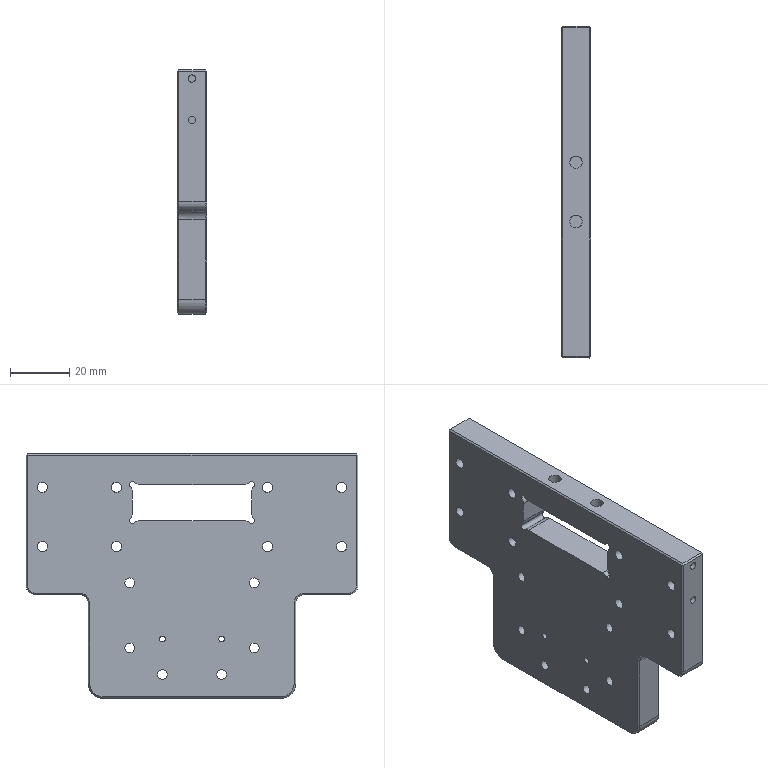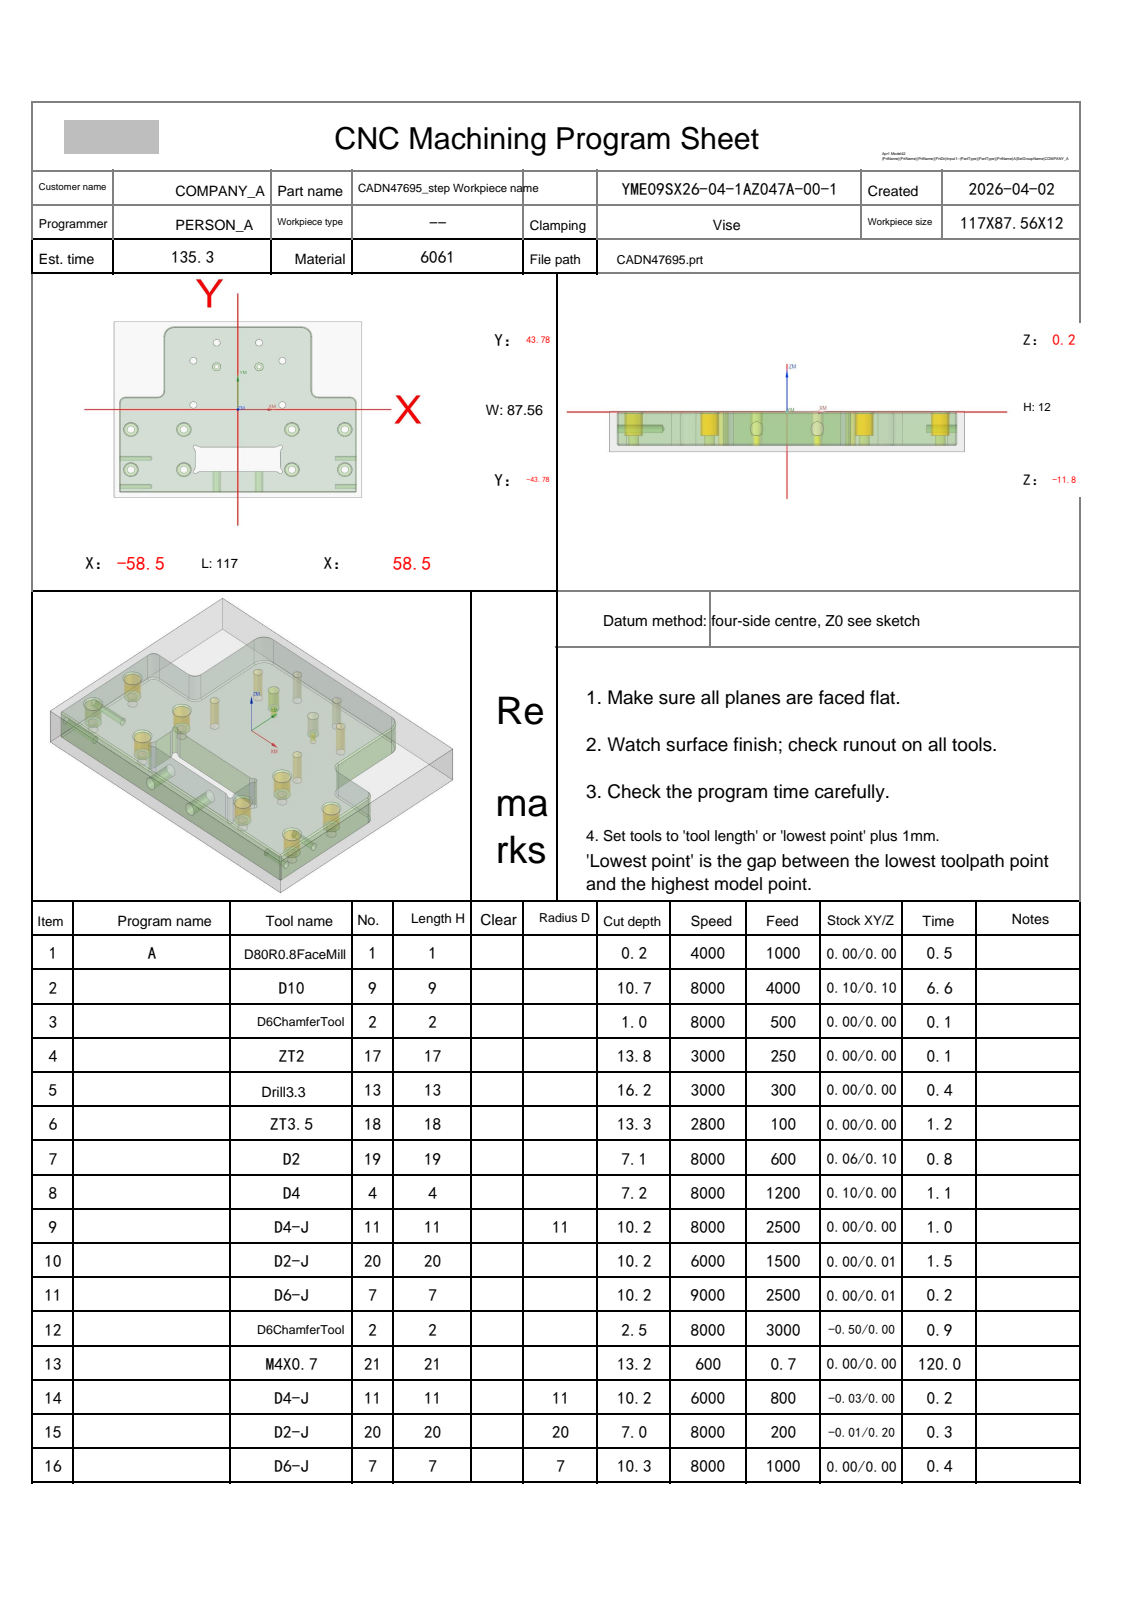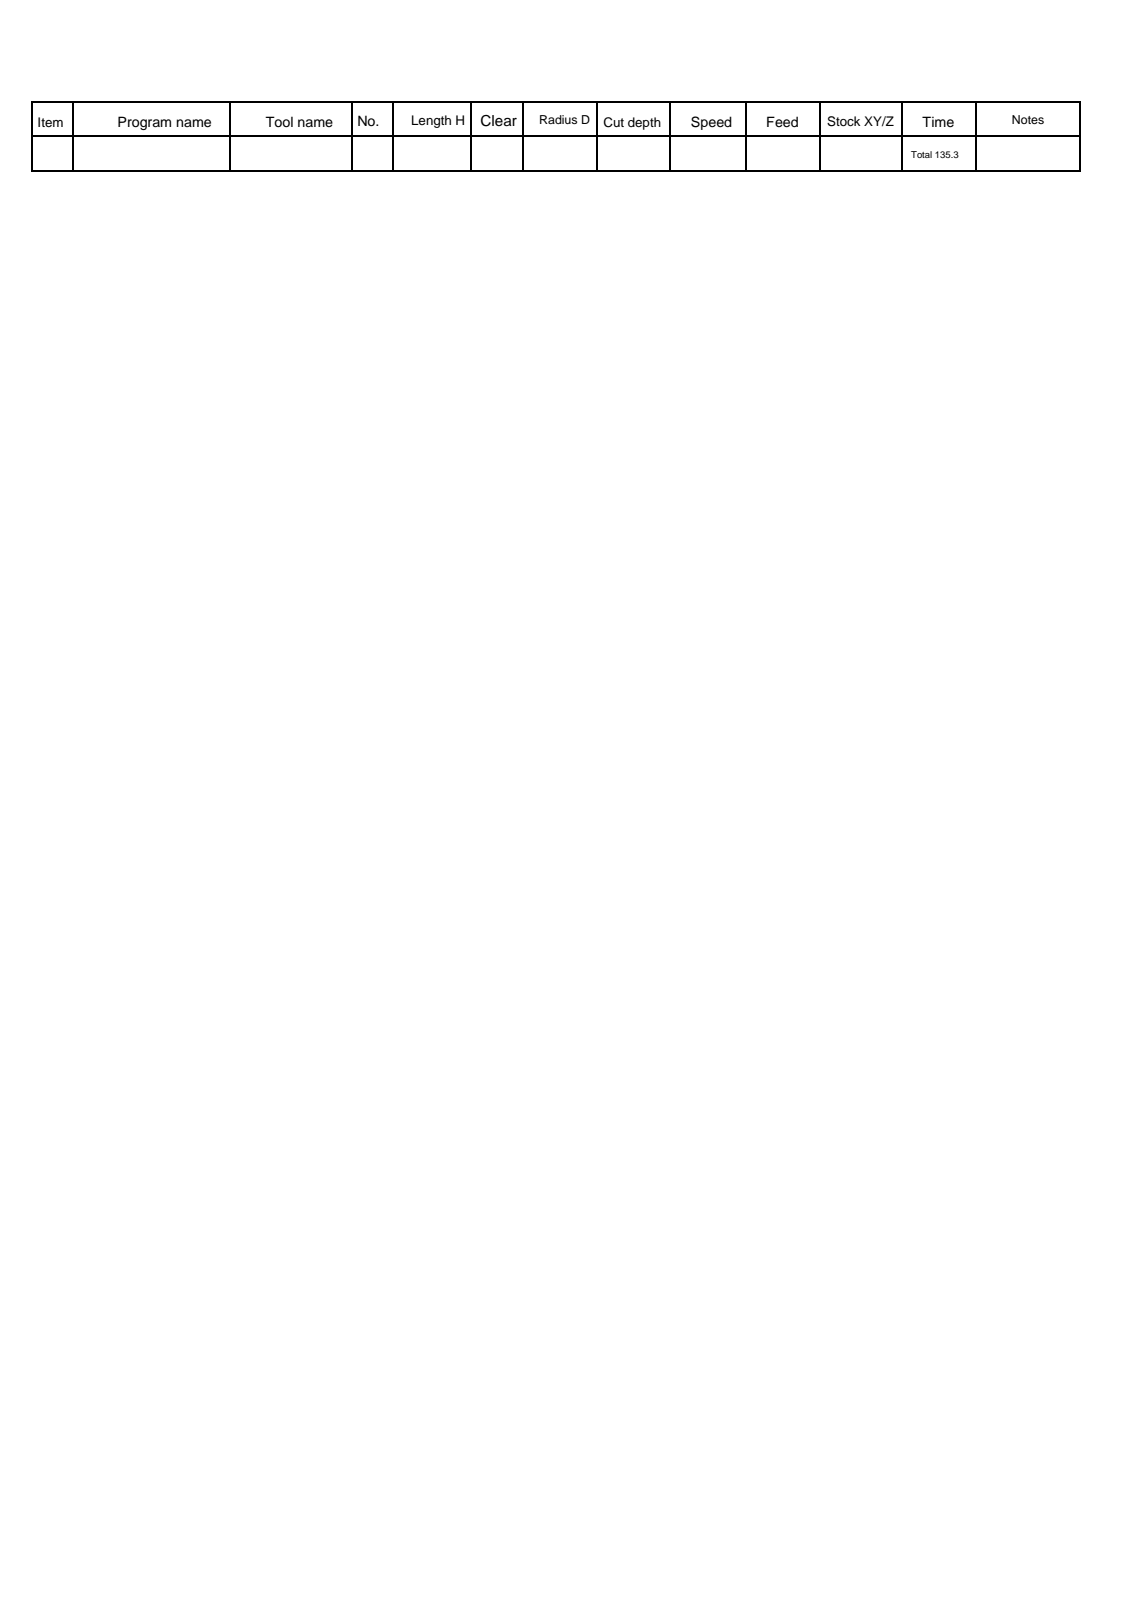NC program | NX | posted by the shop | part box 10 x 112 x 82.562 mm
Lines 3038 to 4053 of 16718:
N9 T11 M06
(D4-J  D=4. R=0. H=11 ce=0.00 di=0.00)
G00 G90 G54 X-50.5 Y-29.931 M03 S8000
G43 H11 Z20.
M08
Z.5
G41 D11
G01 X-50.577 Y-29.747 F500.
G03 X-51.02 Y-29.451 I-.443 J-.185
X-51.5 Y-29.931 I0.0 J-.48
X-51.5 Y-29.931 Z-4.5 I1. J0.0
X-49.5 Y-29.931 Z-7. I1. J0.0
X-50.5 Y-28.931 I-1. J0.0
X-51.5 Y-29.931 I0.0 J-1.
X-50.5 Y-30.931 I1. J0.0
X-49.5 Y-29.931 I0.0 J1.
X-49.98 Y-29.451 I-.48 J0.0
X-50.423 Y-29.747 I0.0 J-.48
G01 G40 X-50.5 Y-29.931
G00 Z20.
Y-9.931
Z.5
G41 D11
G01 X-50.577 Y-9.747
G03 X-51.02 Y-9.451 I-.443 J-.185
X-51.5 Y-9.931 I0.0 J-.48
X-51.5 Y-9.931 Z-4.5 I1. J0.0
X-49.5 Y-9.931 Z-7. I1. J0.0
X-50.5 Y-8.931 I-1. J0.0
X-51.5 Y-9.931 I0.0 J-1.
X-50.5 Y-10.931 I1. J0.0
X-49.5 Y-9.931 I0.0 J1.
X-49.98 Y-9.451 I-.48 J0.0
X-50.423 Y-9.747 I0.0 J-.48
G01 G40 X-50.5 Y-9.931
G00 Z20.
X-25.5
Z.5
G41 D11
G01 X-25.577 Y-9.747
G03 X-26.02 Y-9.451 I-.443 J-.185
X-26.5 Y-9.931 I0.0 J-.48
X-26.5 Y-9.931 Z-4.5 I1. J0.0
X-24.5 Y-9.931 Z-7. I1. J0.0
X-25.5 Y-8.931 I-1. J0.0
X-26.5 Y-9.931 I0.0 J-1.
X-25.5 Y-10.931 I1. J0.0
X-24.5 Y-9.931 I0.0 J1.
X-24.98 Y-9.451 I-.48 J0.0
X-25.423 Y-9.747 I0.0 J-.48
G01 G40 X-25.5 Y-9.931
G00 Z20.
Y-29.931
Z.5
G41 D11
G01 X-25.577 Y-29.747
G03 X-26.02 Y-29.451 I-.443 J-.185
X-26.5 Y-29.931 I0.0 J-.48
X-26.5 Y-29.931 Z-4.5 I1. J0.0
X-24.5 Y-29.931 Z-7. I1. J0.0
X-25.5 Y-28.931 I-1. J0.0
X-26.5 Y-29.931 I0.0 J-1.
X-25.5 Y-30.931 I1. J0.0
X-24.5 Y-29.931 I0.0 J1.
X-24.98 Y-29.451 I-.48 J0.0
X-25.423 Y-29.747 I0.0 J-.48
G01 G40 X-25.5 Y-29.931
G00 Z20.
X25.5
Z.5
G41 D11
G01 X25.423 Y-29.747
G03 X24.98 Y-29.451 I-.443 J-.185
X24.5 Y-29.931 I0.0 J-.48
X24.5 Y-29.931 Z-4.5 I1. J0.0
X26.5 Y-29.931 Z-7. I1. J0.0
X25.5 Y-28.931 I-1. J0.0
X24.5 Y-29.931 I0.0 J-1.
X25.5 Y-30.931 I1. J0.0
X26.5 Y-29.931 I0.0 J1.
X26.02 Y-29.451 I-.48 J0.0
X25.577 Y-29.747 I0.0 J-.48
G01 G40 X25.5 Y-29.931
G00 Z20.
Y-9.931
Z.5
G41 D11
G01 X25.423 Y-9.747
G03 X24.98 Y-9.451 I-.443 J-.185
X24.5 Y-9.931 I0.0 J-.48
X24.5 Y-9.931 Z-4.5 I1. J0.0
X26.5 Y-9.931 Z-7. I1. J0.0
X25.5 Y-8.931 I-1. J0.0
X24.5 Y-9.931 I0.0 J-1.
X25.5 Y-10.931 I1. J0.0
X26.5 Y-9.931 I0.0 J1.
X26.02 Y-9.451 I-.48 J0.0
X25.577 Y-9.747 I0.0 J-.48
G01 G40 X25.5 Y-9.931
G00 Z20.
X50.5
Z.5
G41 D11
G01 X50.423 Y-9.747
G03 X49.98 Y-9.451 I-.443 J-.185
X49.5 Y-9.931 I0.0 J-.48
X49.5 Y-9.931 Z-4.5 I1. J0.0
X51.5 Y-9.931 Z-7. I1. J0.0
X50.5 Y-8.931 I-1. J0.0
X49.5 Y-9.931 I0.0 J-1.
X50.5 Y-10.931 I1. J0.0
X51.5 Y-9.931 I0.0 J1.
X51.02 Y-9.451 I-.48 J0.0
X50.577 Y-9.747 I0.0 J-.48
G01 G40 X50.5 Y-9.931
G00 Z20.
Y-29.931
Z.5
G41 D11
G01 X50.423 Y-29.747
G03 X49.98 Y-29.451 I-.443 J-.185
X49.5 Y-29.931 I0.0 J-.48
X49.5 Y-29.931 Z-4.5 I1. J0.0
X51.5 Y-29.931 Z-7. I1. J0.0
X50.5 Y-28.931 I-1. J0.0
X49.5 Y-29.931 I0.0 J-1.
X50.5 Y-30.931 I1. J0.0
X51.5 Y-29.931 I0.0 J1.
X51.02 Y-29.451 I-.48 J0.0
X50.577 Y-29.747 I0.0 J-.48
G01 G40 X50.5 Y-29.931
G00 Z20.
G00 G90 X14.547 Y-28.28 M03 S6000
Z20.
Z.306
G01 X14.548 Y-28.287 Z.22 F2000.
X14.551 Y-28.306 Z.142
X14.556 Y-28.335 Z.072
X14.564 Y-28.374 Z.01
X14.575 Y-28.419 Z-.046
X14.589 Y-28.47 Z-.095
X14.606 Y-28.525 Z-.137
X14.627 Y-28.581 Z-.174
X14.651 Y-28.637 Z-.205
X14.68 Y-28.691 Z-.231
X14.712 Y-28.742 Z-.252
X14.749 Y-28.787 Z-.268
X14.791 Y-28.826 Z-.28
X14.838 Y-28.855 Z-.288
X14.89 Y-28.874 Z-.293
X14.947 Y-28.881 Z-.294
X17.651 F2500.
G02 X18.125 Y-28.906 I0.0 J-4.5
X18.1 Y-28.432 I4.475 J.475
G01 Y-25.728
X18.084 Y-25.685 Z-.295
X18.038 Y-25.664 Z-.298
X17.966 Y-25.663 Z-.302
X17.87 Y-25.681 Z-.307
X17.755 Y-25.716 Z-.314
X17.624 Y-25.766 Z-.322
X17.48 Y-25.83 Z-.331
X17.327 Y-25.905 Z-.341
X17.086 Y-26.039 Z-.357
X16.847 Y-26.187 Z-.374
X16.509 Y-26.429 Z-.4
X16.194 Y-26.696 Z-.427
X15.903 Y-26.986 Z-.455
X15.636 Y-27.3 Z-.482
X15.395 Y-27.636 Z-.509
X15.294 Y-27.795 Z-.52
X15.201 Y-27.956 Z-.531
X15.116 Y-28.114 Z-.542
X15.042 Y-28.266 Z-.551
X14.98 Y-28.408 Z-.56
X14.931 Y-28.539 Z-.568
X14.897 Y-28.653 Z-.575
X14.881 Y-28.748 Z-.581
X14.882 Y-28.82 Z-.585
X14.904 Y-28.865 Z-.587
X14.947 Y-28.881 Z-.588
X17.651
G02 X18.125 Y-28.906 I0.0 J-4.5
X18.1 Y-28.432 I4.475 J.475
G01 Y-25.728
X18.084 Y-25.685 Z-.589
X18.038 Y-25.664 Z-.592
X17.966 Y-25.663 Z-.596
X17.87 Y-25.681 Z-.601
X17.755 Y-25.716 Z-.608
X17.624 Y-25.766 Z-.616
X17.48 Y-25.83 Z-.625
X17.327 Y-25.905 Z-.635
X17.086 Y-26.039 Z-.651
X16.847 Y-26.187 Z-.668
X16.509 Y-26.429 Z-.694
X16.194 Y-26.696 Z-.722
X15.903 Y-26.986 Z-.749
X15.636 Y-27.3 Z-.776
X15.395 Y-27.636 Z-.803
X15.294 Y-27.795 Z-.814
X15.201 Y-27.956 Z-.825
X15.116 Y-28.114 Z-.836
X15.042 Y-28.266 Z-.846
X14.98 Y-28.408 Z-.855
X14.931 Y-28.539 Z-.862
X14.897 Y-28.653 Z-.869
X14.881 Y-28.748 Z-.875
X14.882 Y-28.82 Z-.879
X14.904 Y-28.865 Z-.881
X14.947 Y-28.881 Z-.882
X17.651
G02 X18.125 Y-28.906 I0.0 J-4.5
X18.1 Y-28.432 I4.475 J.475
G01 Y-25.728
X18.084 Y-25.685 Z-.883
X18.038 Y-25.664 Z-.886
X17.966 Y-25.663 Z-.89
X17.87 Y-25.681 Z-.895
X17.755 Y-25.716 Z-.902
X17.624 Y-25.766 Z-.91
X17.48 Y-25.83 Z-.919
X17.327 Y-25.905 Z-.929
X17.086 Y-26.039 Z-.945
X16.847 Y-26.187 Z-.962
X16.509 Y-26.429 Z-.988
X16.194 Y-26.696 Z-1.016
X15.903 Y-26.986 Z-1.043
X15.636 Y-27.3 Z-1.07
X15.395 Y-27.636 Z-1.097
X15.294 Y-27.795 Z-1.108
X15.201 Y-27.956 Z-1.119
X15.116 Y-28.114 Z-1.13
X15.042 Y-28.266 Z-1.14
X14.98 Y-28.408 Z-1.149
X14.931 Y-28.539 Z-1.157
X14.897 Y-28.653 Z-1.163
X14.881 Y-28.748 Z-1.169
X14.882 Y-28.82 Z-1.173
X14.904 Y-28.865 Z-1.176
X14.947 Y-28.881
X17.651
G02 X18.125 Y-28.906 I0.0 J-4.5
X18.1 Y-28.432 I4.475 J.475
G01 Y-25.728
X18.084 Y-25.685 Z-1.177
X18.038 Y-25.664 Z-1.18
X17.966 Y-25.663 Z-1.184
X17.87 Y-25.681 Z-1.19
X17.755 Y-25.716 Z-1.196
X17.624 Y-25.766 Z-1.204
X17.48 Y-25.83 Z-1.213
X17.327 Y-25.905 Z-1.223
X17.086 Y-26.039 Z-1.239
X16.847 Y-26.187 Z-1.256
X16.509 Y-26.429 Z-1.283
X16.194 Y-26.696 Z-1.31
X15.903 Y-26.986 Z-1.337
X15.636 Y-27.3 Z-1.365
X15.395 Y-27.636 Z-1.391
X15.294 Y-27.795 Z-1.402
X15.201 Y-27.956 Z-1.414
X15.116 Y-28.114 Z-1.424
X15.042 Y-28.266 Z-1.434
X14.98 Y-28.408 Z-1.443
X14.931 Y-28.539 Z-1.451
X14.897 Y-28.653 Z-1.457
X14.881 Y-28.748 Z-1.463
X14.882 Y-28.82 Z-1.467
X14.904 Y-28.865 Z-1.47
X14.947 Y-28.881 Z-1.471
X17.651
G02 X18.125 Y-28.906 I0.0 J-4.5
X18.1 Y-28.432 I4.475 J.475
G01 Y-25.728
X18.084 Y-25.685
X18.038 Y-25.664 Z-1.474
X17.966 Y-25.663 Z-1.478
X17.87 Y-25.681 Z-1.484
X17.755 Y-25.716 Z-1.491
X17.624 Y-25.766 Z-1.498
X17.48 Y-25.83 Z-1.507
X17.327 Y-25.905 Z-1.517
X17.086 Y-26.039 Z-1.533
X16.847 Y-26.187 Z-1.55
X16.509 Y-26.429 Z-1.577
X16.194 Y-26.696 Z-1.604
X15.903 Y-26.986 Z-1.631
X15.636 Y-27.3 Z-1.659
X15.395 Y-27.636 Z-1.685
X15.294 Y-27.795 Z-1.697
X15.201 Y-27.956 Z-1.708
X15.116 Y-28.114 Z-1.718
X15.042 Y-28.266 Z-1.728
X14.98 Y-28.408 Z-1.737
X14.931 Y-28.539 Z-1.745
X14.897 Y-28.653 Z-1.752
X14.881 Y-28.748 Z-1.757
X14.882 Y-28.82 Z-1.761
X14.904 Y-28.865 Z-1.764
X14.947 Y-28.881 Z-1.765
X17.651
G02 X18.125 Y-28.906 I0.0 J-4.5
X18.1 Y-28.432 I4.475 J.475
G01 Y-25.728
X18.084 Y-25.685 Z-1.766
X18.038 Y-25.664 Z-1.768
X17.966 Y-25.663 Z-1.772
X17.87 Y-25.681 Z-1.778
X17.755 Y-25.716 Z-1.785
X17.624 Y-25.766 Z-1.793
X17.48 Y-25.83 Z-1.801
X17.327 Y-25.905 Z-1.811
X17.086 Y-26.039 Z-1.827
X16.847 Y-26.187 Z-1.844
X16.509 Y-26.429 Z-1.871
X16.194 Y-26.696 Z-1.898
X15.903 Y-26.986 Z-1.926
X15.636 Y-27.3 Z-1.953
X15.395 Y-27.636 Z-1.979
X15.294 Y-27.795 Z-1.991
X15.201 Y-27.956 Z-2.002
X15.116 Y-28.114 Z-2.012
X15.042 Y-28.266 Z-2.022
X14.98 Y-28.408 Z-2.031
X14.931 Y-28.539 Z-2.039
X14.897 Y-28.653 Z-2.046
X14.881 Y-28.748 Z-2.051
X14.882 Y-28.82 Z-2.055
X14.904 Y-28.865 Z-2.058
X14.947 Y-28.881 Z-2.059
X17.651
G02 X18.125 Y-28.906 I0.0 J-4.5
X18.1 Y-28.432 I4.475 J.475
G01 Y-25.728
X18.084 Y-25.685 Z-2.06
X18.038 Y-25.664 Z-2.062
X17.966 Y-25.663 Z-2.066
X17.87 Y-25.681 Z-2.072
X17.755 Y-25.716 Z-2.079
X17.624 Y-25.766 Z-2.087
X17.48 Y-25.83 Z-2.096
X17.327 Y-25.905 Z-2.105
X17.086 Y-26.039 Z-2.122
X16.847 Y-26.187 Z-2.138
X16.509 Y-26.429 Z-2.165
X16.194 Y-26.696 Z-2.192
X15.903 Y-26.986 Z-2.22
X15.636 Y-27.3 Z-2.247
X15.395 Y-27.636 Z-2.273
X15.294 Y-27.795 Z-2.285
X15.201 Y-27.956 Z-2.296
X15.116 Y-28.114 Z-2.306
X15.042 Y-28.266 Z-2.316
X14.98 Y-28.408 Z-2.325
X14.931 Y-28.539 Z-2.333
X14.897 Y-28.653 Z-2.34
X14.881 Y-28.748 Z-2.345
X14.882 Y-28.82 Z-2.349
X14.904 Y-28.865 Z-2.352
X14.947 Y-28.881 Z-2.353
X17.651
G02 X18.125 Y-28.906 I0.0 J-4.5
X18.1 Y-28.432 I4.475 J.475
G01 Y-25.728
X18.084 Y-25.685 Z-2.354
X18.038 Y-25.664 Z-2.356
X17.966 Y-25.663 Z-2.361
X17.87 Y-25.681 Z-2.366
X17.755 Y-25.716 Z-2.373
X17.624 Y-25.766 Z-2.381
X17.48 Y-25.83 Z-2.39
X17.327 Y-25.905 Z-2.399
X17.086 Y-26.039 Z-2.416
X16.847 Y-26.187 Z-2.433
X16.509 Y-26.429 Z-2.459
X16.194 Y-26.696 Z-2.486
X15.903 Y-26.986 Z-2.514
X15.636 Y-27.3 Z-2.541
X15.395 Y-27.636 Z-2.567
X15.294 Y-27.795 Z-2.579
X15.201 Y-27.956 Z-2.59
X15.116 Y-28.114 Z-2.601
X15.042 Y-28.266 Z-2.61
X14.98 Y-28.408 Z-2.619
X14.931 Y-28.539 Z-2.627
X14.897 Y-28.653 Z-2.634
X14.881 Y-28.748 Z-2.639
X14.882 Y-28.82 Z-2.644
X14.904 Y-28.865 Z-2.646
X14.947 Y-28.881 Z-2.647
X17.651
G02 X18.125 Y-28.906 I0.0 J-4.5
X18.1 Y-28.432 I4.475 J.475
G01 Y-25.728
X18.084 Y-25.685 Z-2.648
X18.038 Y-25.664 Z-2.651
X17.966 Y-25.663 Z-2.655
X17.87 Y-25.681 Z-2.66
X17.755 Y-25.716 Z-2.667
X17.624 Y-25.766 Z-2.675
X17.48 Y-25.83 Z-2.684
X17.327 Y-25.905 Z-2.694
X17.086 Y-26.039 Z-2.71
X16.847 Y-26.187 Z-2.727
X16.509 Y-26.429 Z-2.753
X16.194 Y-26.696 Z-2.78
X15.903 Y-26.986 Z-2.808
X15.636 Y-27.3 Z-2.835
X15.395 Y-27.636 Z-2.862
X15.294 Y-27.795 Z-2.873
X15.201 Y-27.956 Z-2.884
X15.116 Y-28.114 Z-2.895
X15.042 Y-28.266 Z-2.904
X14.98 Y-28.408 Z-2.913
X14.931 Y-28.539 Z-2.921
X14.897 Y-28.653 Z-2.928
X14.881 Y-28.748 Z-2.934
X14.882 Y-28.82 Z-2.938
X14.904 Y-28.865 Z-2.94
X14.947 Y-28.881 Z-2.941
X17.651
G02 X18.125 Y-28.906 I0.0 J-4.5
X18.1 Y-28.432 I4.475 J.475
G01 Y-25.728
X18.084 Y-25.685 Z-2.942
X18.038 Y-25.664 Z-2.945
X17.966 Y-25.663 Z-2.949
X17.87 Y-25.681 Z-2.954
X17.755 Y-25.716 Z-2.961
X17.624 Y-25.766 Z-2.969
X17.48 Y-25.83 Z-2.978
X17.327 Y-25.905 Z-2.988
X17.086 Y-26.039 Z-3.004
X16.847 Y-26.187 Z-3.021
X16.509 Y-26.429 Z-3.047
X16.194 Y-26.696 Z-3.074
X15.903 Y-26.986 Z-3.102
X15.636 Y-27.3 Z-3.129
X15.395 Y-27.636 Z-3.156
X15.294 Y-27.795 Z-3.167
X15.201 Y-27.956 Z-3.178
X15.116 Y-28.114 Z-3.189
X15.042 Y-28.266 Z-3.199
X14.98 Y-28.408 Z-3.207
X14.931 Y-28.539 Z-3.215
X14.897 Y-28.653 Z-3.222
X14.881 Y-28.748 Z-3.228
X14.882 Y-28.82 Z-3.232
X14.904 Y-28.865 Z-3.234
X14.947 Y-28.881 Z-3.235
X17.651
G02 X18.125 Y-28.906 I0.0 J-4.5
X18.1 Y-28.432 I4.475 J.475
G01 Y-25.728
X18.084 Y-25.685 Z-3.236
X18.038 Y-25.664 Z-3.239
X17.966 Y-25.663 Z-3.243
X17.87 Y-25.681 Z-3.248
X17.755 Y-25.716 Z-3.255
X17.624 Y-25.766 Z-3.263
X17.48 Y-25.83 Z-3.272
X17.327 Y-25.905 Z-3.282
X17.086 Y-26.039 Z-3.298
X16.847 Y-26.187 Z-3.315
X16.509 Y-26.429 Z-3.341
X16.194 Y-26.696 Z-3.369
X15.903 Y-26.986 Z-3.396
X15.636 Y-27.3 Z-3.423
X15.395 Y-27.636 Z-3.45
X15.294 Y-27.795 Z-3.461
X15.201 Y-27.956 Z-3.472
X15.116 Y-28.114 Z-3.483
X15.042 Y-28.266 Z-3.493
X14.98 Y-28.408 Z-3.502
X14.931 Y-28.539 Z-3.51
X14.897 Y-28.653 Z-3.516
X14.881 Y-28.748 Z-3.522
X14.882 Y-28.82 Z-3.526
X14.904 Y-28.865 Z-3.529
X14.947 Y-28.881
X17.651
G02 X18.125 Y-28.906 I0.0 J-4.5
X18.1 Y-28.432 I4.475 J.475
G01 Y-25.728
X18.084 Y-25.685 Z-3.53
X18.038 Y-25.664 Z-3.533
X17.966 Y-25.663 Z-3.537
X17.87 Y-25.681 Z-3.543
X17.755 Y-25.716 Z-3.549
X17.624 Y-25.766 Z-3.557
X17.48 Y-25.83 Z-3.566
X17.327 Y-25.905 Z-3.576
X17.086 Y-26.039 Z-3.592
X16.847 Y-26.187 Z-3.609
X16.509 Y-26.429 Z-3.635
X16.194 Y-26.696 Z-3.663
X15.903 Y-26.986 Z-3.69
X15.636 Y-27.3 Z-3.718
X15.395 Y-27.636 Z-3.744
X15.294 Y-27.795 Z-3.755
X15.201 Y-27.956 Z-3.766
X15.116 Y-28.114 Z-3.777
X15.042 Y-28.266 Z-3.787
X14.98 Y-28.408 Z-3.796
X14.931 Y-28.539 Z-3.804
X14.897 Y-28.653 Z-3.81
X14.881 Y-28.748 Z-3.816
X14.882 Y-28.82 Z-3.82
X14.904 Y-28.865 Z-3.823
X14.947 Y-28.881 Z-3.824
X17.651
G02 X18.125 Y-28.906 I0.0 J-4.5
X18.1 Y-28.432 I4.475 J.475
G01 Y-25.728
X18.084 Y-25.685
X18.038 Y-25.664 Z-3.827
X17.966 Y-25.663 Z-3.831
X17.87 Y-25.681 Z-3.837
X17.755 Y-25.716 Z-3.843
X17.624 Y-25.766 Z-3.851
X17.48 Y-25.83 Z-3.86
X17.327 Y-25.905 Z-3.87
X17.086 Y-26.039 Z-3.886
X16.847 Y-26.187 Z-3.903
X16.509 Y-26.429 Z-3.93
X16.194 Y-26.696 Z-3.957
X15.903 Y-26.986 Z-3.984
X15.636 Y-27.3 Z-4.012
X15.395 Y-27.636 Z-4.038
X15.294 Y-27.795 Z-4.05
X15.201 Y-27.956 Z-4.061
X15.116 Y-28.114 Z-4.071
X15.042 Y-28.266 Z-4.081
X14.98 Y-28.408 Z-4.09
X14.931 Y-28.539 Z-4.098
X14.897 Y-28.653 Z-4.105
X14.881 Y-28.748 Z-4.11
X14.882 Y-28.82 Z-4.114
X14.904 Y-28.865 Z-4.117
X14.947 Y-28.881 Z-4.118
X17.651
G02 X18.125 Y-28.906 I0.0 J-4.5
X18.1 Y-28.432 I4.475 J.475
G01 Y-25.728
X18.084 Y-25.685 Z-4.119
X18.038 Y-25.664 Z-4.121
X17.966 Y-25.663 Z-4.125
X17.87 Y-25.681 Z-4.131
X17.755 Y-25.716 Z-4.138
X17.624 Y-25.766 Z-4.145
X17.48 Y-25.83 Z-4.154
X17.327 Y-25.905 Z-4.164
X17.086 Y-26.039 Z-4.18
X16.847 Y-26.187 Z-4.197
X16.509 Y-26.429 Z-4.224
X16.194 Y-26.696 Z-4.251
X15.903 Y-26.986 Z-4.278
X15.636 Y-27.3 Z-4.306
X15.395 Y-27.636 Z-4.332
X15.294 Y-27.795 Z-4.344
X15.201 Y-27.956 Z-4.355
X15.116 Y-28.114 Z-4.365
X15.042 Y-28.266 Z-4.375
X14.98 Y-28.408 Z-4.384
X14.931 Y-28.539 Z-4.392
X14.897 Y-28.653 Z-4.399
X14.881 Y-28.748 Z-4.404
X14.882 Y-28.82 Z-4.408
X14.904 Y-28.865 Z-4.411
X14.947 Y-28.881 Z-4.412
X17.651
G02 X18.125 Y-28.906 I0.0 J-4.5
X18.1 Y-28.432 I4.475 J.475
G01 Y-25.728
X18.084 Y-25.685 Z-4.413
X18.038 Y-25.664 Z-4.415
X17.966 Y-25.663 Z-4.419
X17.87 Y-25.681 Z-4.425
X17.755 Y-25.716 Z-4.432
X17.624 Y-25.766 Z-4.44
X17.48 Y-25.83 Z-4.449
X17.327 Y-25.905 Z-4.458
X17.086 Y-26.039 Z-4.474
X16.847 Y-26.187 Z-4.491
X16.509 Y-26.429 Z-4.518
X16.194 Y-26.696 Z-4.545
X15.903 Y-26.986 Z-4.573
X15.636 Y-27.3 Z-4.6
X15.395 Y-27.636 Z-4.626
X15.294 Y-27.795 Z-4.638
X15.201 Y-27.956 Z-4.649
X15.116 Y-28.114 Z-4.659
X15.042 Y-28.266 Z-4.669
X14.98 Y-28.408 Z-4.678
X14.931 Y-28.539 Z-4.686
X14.897 Y-28.653 Z-4.693
X14.881 Y-28.748 Z-4.698
X14.882 Y-28.82 Z-4.702
X14.904 Y-28.865 Z-4.705
X14.947 Y-28.881 Z-4.706
X17.651
G02 X18.125 Y-28.906 I0.0 J-4.5
X18.1 Y-28.432 I4.475 J.475
G01 Y-25.728
X18.084 Y-25.685 Z-4.707
X18.038 Y-25.664 Z-4.709
X17.966 Y-25.663 Z-4.713
X17.87 Y-25.681 Z-4.719
X17.755 Y-25.716 Z-4.726
X17.624 Y-25.766 Z-4.734
X17.48 Y-25.83 Z-4.743
X17.327 Y-25.905 Z-4.752
X17.086 Y-26.039 Z-4.769
X16.847 Y-26.187 Z-4.786
X16.509 Y-26.429 Z-4.812
X16.194 Y-26.696 Z-4.839
X15.903 Y-26.986 Z-4.867
X15.636 Y-27.3 Z-4.894
X15.395 Y-27.636 Z-4.92
X15.294 Y-27.795 Z-4.932
X15.201 Y-27.956 Z-4.943
X15.116 Y-28.114 Z-4.953
X15.042 Y-28.266 Z-4.963
X14.98 Y-28.408 Z-4.972
X14.931 Y-28.539 Z-4.98
X14.897 Y-28.653 Z-4.987
X14.881 Y-28.748 Z-4.992
X14.882 Y-28.82 Z-4.997
X14.904 Y-28.865 Z-4.999
X14.947 Y-28.881 Z-5.
X17.651
G02 X18.125 Y-28.906 I0.0 J-4.5
X18.1 Y-28.432 I4.475 J.475
G01 Y-25.728
X18.084 Y-25.685 Z-5.001
X18.038 Y-25.664 Z-5.003
X17.966 Y-25.663 Z-5.008
X17.87 Y-25.681 Z-5.013
X17.755 Y-25.716 Z-5.02
X17.624 Y-25.766 Z-5.028
X17.48 Y-25.83 Z-5.037
X17.327 Y-25.905 Z-5.047
X17.086 Y-26.039 Z-5.063
X16.847 Y-26.187 Z-5.08
X16.509 Y-26.429 Z-5.106
X16.194 Y-26.696 Z-5.133
X15.903 Y-26.986 Z-5.161
X15.636 Y-27.3 Z-5.188
X15.395 Y-27.636 Z-5.214
X15.294 Y-27.795 Z-5.226
X15.201 Y-27.956 Z-5.237
X15.116 Y-28.114 Z-5.248
X15.042 Y-28.266 Z-5.257
X14.98 Y-28.408 Z-5.266
X14.931 Y-28.539 Z-5.274
X14.897 Y-28.653 Z-5.281
X14.881 Y-28.748 Z-5.287
X14.882 Y-28.82 Z-5.291
X14.904 Y-28.865 Z-5.293
X14.947 Y-28.881 Z-5.294
X17.651
G02 X18.125 Y-28.906 I0.0 J-4.5
X18.1 Y-28.432 I4.475 J.475
G01 Y-25.728
X18.084 Y-25.685 Z-5.295
X18.038 Y-25.664 Z-5.298
X17.966 Y-25.663 Z-5.302
X17.87 Y-25.681 Z-5.307
X17.755 Y-25.716 Z-5.314
X17.624 Y-25.766 Z-5.322
X17.48 Y-25.83 Z-5.331
X17.327 Y-25.905 Z-5.341
X17.086 Y-26.039 Z-5.357
X16.847 Y-26.187 Z-5.374
X16.509 Y-26.429 Z-5.4
X16.194 Y-26.696 Z-5.427
X15.903 Y-26.986 Z-5.455
X15.636 Y-27.3 Z-5.482
X15.395 Y-27.636 Z-5.509
X15.294 Y-27.795 Z-5.52
X15.201 Y-27.956 Z-5.531
X15.116 Y-28.114 Z-5.542
X15.042 Y-28.266 Z-5.551
X14.98 Y-28.408 Z-5.56
X14.931 Y-28.539 Z-5.568
X14.897 Y-28.653 Z-5.575
X14.881 Y-28.748 Z-5.581
X14.882 Y-28.82 Z-5.585
X14.904 Y-28.865 Z-5.587
X14.947 Y-28.881 Z-5.588
X17.651
G02 X18.125 Y-28.906 I0.0 J-4.5
X18.1 Y-28.432 I4.475 J.475
G01 Y-25.728
X18.084 Y-25.685 Z-5.589
X18.038 Y-25.664 Z-5.592
X17.966 Y-25.663 Z-5.596
X17.87 Y-25.681 Z-5.601
X17.755 Y-25.716 Z-5.608
X17.624 Y-25.766 Z-5.616
X17.48 Y-25.83 Z-5.625
X17.327 Y-25.905 Z-5.635
X17.086 Y-26.039 Z-5.651
X16.847 Y-26.187 Z-5.668
X16.509 Y-26.429 Z-5.694
X16.194 Y-26.696 Z-5.722
X15.903 Y-26.986 Z-5.749
X15.636 Y-27.3 Z-5.776
X15.395 Y-27.636 Z-5.803
X15.294 Y-27.795 Z-5.814
X15.201 Y-27.956 Z-5.825
X15.116 Y-28.114 Z-5.836
X15.042 Y-28.266 Z-5.846
X14.98 Y-28.408 Z-5.855
X14.931 Y-28.539 Z-5.862
X14.897 Y-28.653 Z-5.869
X14.881 Y-28.748 Z-5.875
X14.882 Y-28.82 Z-5.879
X14.904 Y-28.865 Z-5.881
X14.947 Y-28.881 Z-5.882
X17.651
G02 X18.125 Y-28.906 I0.0 J-4.5
X18.1 Y-28.432 I4.475 J.475
G01 Y-25.728
X18.084 Y-25.685 Z-5.883
X18.038 Y-25.664 Z-5.886
X17.966 Y-25.663 Z-5.89
X17.87 Y-25.681 Z-5.895
X17.755 Y-25.716 Z-5.902
X17.624 Y-25.766 Z-5.91
X17.48 Y-25.83 Z-5.919
X17.327 Y-25.905 Z-5.929
X17.086 Y-26.039 Z-5.945
X16.847 Y-26.187 Z-5.962
X16.509 Y-26.429 Z-5.988
X16.194 Y-26.696 Z-6.016
X15.903 Y-26.986 Z-6.043
X15.636 Y-27.3 Z-6.07
X15.395 Y-27.636 Z-6.097
X15.294 Y-27.795 Z-6.108
X15.201 Y-27.956 Z-6.119
X15.116 Y-28.114 Z-6.13
X15.042 Y-28.266 Z-6.14
X14.98 Y-28.408 Z-6.149
X14.931 Y-28.539 Z-6.157
X14.897 Y-28.653 Z-6.163
X14.881 Y-28.748 Z-6.169
X14.882 Y-28.82 Z-6.173
X14.904 Y-28.865 Z-6.176
X14.947 Y-28.881
X17.651
G02 X18.125 Y-28.906 I0.0 J-4.5
X18.1 Y-28.432 I4.475 J.475
G01 Y-25.728
X18.084 Y-25.685 Z-6.177
X18.038 Y-25.664 Z-6.18
X17.966 Y-25.663 Z-6.184
X17.87 Y-25.681 Z-6.19
X17.755 Y-25.716 Z-6.196
X17.624 Y-25.766 Z-6.204
X17.48 Y-25.83 Z-6.213
X17.327 Y-25.905 Z-6.223
X17.086 Y-26.039 Z-6.239
X16.847 Y-26.187 Z-6.256
X16.509 Y-26.429 Z-6.283
X16.194 Y-26.696 Z-6.31
X15.903 Y-26.986 Z-6.337
X15.636 Y-27.3 Z-6.365
X15.395 Y-27.636 Z-6.391
X15.294 Y-27.795 Z-6.402
X15.201 Y-27.956 Z-6.414
X15.116 Y-28.114 Z-6.424
X15.042 Y-28.266 Z-6.434
X14.98 Y-28.408 Z-6.443
X14.931 Y-28.539 Z-6.451
X14.897 Y-28.653 Z-6.457
X14.881 Y-28.748 Z-6.463
X14.882 Y-28.82 Z-6.467
X14.904 Y-28.865 Z-6.47
X14.947 Y-28.881 Z-6.471
X17.651
G02 X18.125 Y-28.906 I0.0 J-4.5
X18.1 Y-28.432 I4.475 J.475
G01 Y-25.728
X18.084 Y-25.685
X18.038 Y-25.664 Z-6.474
X17.966 Y-25.663 Z-6.478
X17.87 Y-25.681 Z-6.484
X17.755 Y-25.716 Z-6.491
X17.624 Y-25.766 Z-6.498
X17.48 Y-25.83 Z-6.507
X17.327 Y-25.905 Z-6.517
X17.086 Y-26.039 Z-6.533
X16.847 Y-26.187 Z-6.55
X16.509 Y-26.429 Z-6.577
X16.194 Y-26.696 Z-6.604
X15.903 Y-26.986 Z-6.631
X15.636 Y-27.3 Z-6.659
X15.395 Y-27.636 Z-6.685
X15.294 Y-27.795 Z-6.697
X15.201 Y-27.956 Z-6.708
X15.116 Y-28.114 Z-6.718
X15.042 Y-28.266 Z-6.728
X14.98 Y-28.408 Z-6.737
X14.931 Y-28.539 Z-6.745
X14.897 Y-28.653 Z-6.752
X14.881 Y-28.748 Z-6.757
X14.882 Y-28.82 Z-6.761
X14.904 Y-28.865 Z-6.764
X14.947 Y-28.881 Z-6.765
X17.651
G02 X18.125 Y-28.906 I0.0 J-4.5
X18.1 Y-28.432 I4.475 J.475
G01 Y-25.728
X18.084 Y-25.685 Z-6.766
X18.038 Y-25.664 Z-6.768
X17.966 Y-25.663 Z-6.772
X17.87 Y-25.681 Z-6.778
X17.755 Y-25.716 Z-6.785
X17.624 Y-25.766 Z-6.793
X17.48 Y-25.83 Z-6.801
X17.327 Y-25.905 Z-6.811
X17.086 Y-26.039 Z-6.827
X16.847 Y-26.187 Z-6.844
X16.509 Y-26.429 Z-6.871
X16.194 Y-26.696 Z-6.898
X15.903 Y-26.986 Z-6.926
X15.636 Y-27.3 Z-6.953
X15.395 Y-27.636 Z-6.979
X15.294 Y-27.795 Z-6.991
X15.201 Y-27.956 Z-7.002
X15.116 Y-28.114 Z-7.012
X15.042 Y-28.266 Z-7.022
X14.98 Y-28.408 Z-7.031
X14.931 Y-28.539 Z-7.039
X14.897 Y-28.653 Z-7.046
X14.881 Y-28.748 Z-7.051
X14.882 Y-28.82 Z-7.055
X14.904 Y-28.865 Z-7.058
X14.947 Y-28.881 Z-7.059
X17.651
G02 X18.125 Y-28.906 I0.0 J-4.5
X18.1 Y-28.432 I4.475 J.475
G01 Y-25.728
X18.084 Y-25.685 Z-7.06
X18.038 Y-25.664 Z-7.062
X17.966 Y-25.663 Z-7.066
X17.87 Y-25.681 Z-7.072
X17.755 Y-25.716 Z-7.079
X17.624 Y-25.766 Z-7.087
X17.48 Y-25.83 Z-7.096
X17.327 Y-25.905 Z-7.105
X17.086 Y-26.039 Z-7.122
X16.847 Y-26.187 Z-7.138
X16.509 Y-26.429 Z-7.165
X16.194 Y-26.696 Z-7.192
X15.903 Y-26.986 Z-7.22
X15.636 Y-27.3 Z-7.247
X15.395 Y-27.636 Z-7.273
X15.294 Y-27.795 Z-7.285
X15.201 Y-27.956 Z-7.296
X15.116 Y-28.114 Z-7.306
X15.042 Y-28.266 Z-7.316
X14.98 Y-28.408 Z-7.325
X14.931 Y-28.539 Z-7.333
X14.897 Y-28.653 Z-7.34
X14.881 Y-28.748 Z-7.345
X14.882 Y-28.82 Z-7.349
X14.904 Y-28.865 Z-7.352
X14.947 Y-28.881 Z-7.353
X17.651
G02 X18.125 Y-28.906 I0.0 J-4.5
X18.1 Y-28.432 I4.475 J.475
G01 Y-25.728
X18.084 Y-25.685 Z-7.354
X18.038 Y-25.664 Z-7.356
X17.966 Y-25.663 Z-7.361
X17.87 Y-25.681 Z-7.366
X17.755 Y-25.716 Z-7.373
X17.624 Y-25.766 Z-7.381
X17.48 Y-25.83 Z-7.39
X17.327 Y-25.905 Z-7.399
X17.086 Y-26.039 Z-7.416
X16.847 Y-26.187 Z-7.433
X16.509 Y-26.429 Z-7.459
X16.194 Y-26.696 Z-7.486
X15.903 Y-26.986 Z-7.514
X15.636 Y-27.3 Z-7.541
X15.395 Y-27.636 Z-7.567
X15.294 Y-27.795 Z-7.579
X15.201 Y-27.956 Z-7.59
X15.116 Y-28.114 Z-7.601
X15.042 Y-28.266 Z-7.61
X14.98 Y-28.408 Z-7.619
X14.931 Y-28.539 Z-7.627
X14.897 Y-28.653 Z-7.634
X14.881 Y-28.748 Z-7.639
X14.882 Y-28.82 Z-7.644
X14.904 Y-28.865 Z-7.646
X14.947 Y-28.881 Z-7.647
X17.651
G02 X18.125 Y-28.906 I0.0 J-4.5
X18.1 Y-28.432 I4.475 J.475
G01 Y-25.728
X18.084 Y-25.685 Z-7.648
X18.038 Y-25.664 Z-7.651
X17.966 Y-25.663 Z-7.655
X17.87 Y-25.681 Z-7.66
X17.755 Y-25.716 Z-7.667
X17.624 Y-25.766 Z-7.675
X17.48 Y-25.83 Z-7.684
X17.327 Y-25.905 Z-7.694
X17.086 Y-26.039 Z-7.71
X16.847 Y-26.187 Z-7.727
X16.509 Y-26.429 Z-7.753
X16.194 Y-26.696 Z-7.78
X15.903 Y-26.986 Z-7.808
X15.636 Y-27.3 Z-7.835
X15.395 Y-27.636 Z-7.862
X15.294 Y-27.795 Z-7.873
X15.201 Y-27.956 Z-7.884
X15.116 Y-28.114 Z-7.895
X15.042 Y-28.266 Z-7.904
X14.98 Y-28.408 Z-7.913
X14.931 Y-28.539 Z-7.921
X14.897 Y-28.653 Z-7.928
X14.881 Y-28.748 Z-7.934
X14.882 Y-28.82 Z-7.938
X14.904 Y-28.865 Z-7.94
X14.947 Y-28.881 Z-7.941
X17.651
G02 X18.125 Y-28.906 I0.0 J-4.5
X18.1 Y-28.432 I4.475 J.475
G01 Y-25.728
X18.084 Y-25.685 Z-7.942
X18.038 Y-25.664 Z-7.945
X17.966 Y-25.663 Z-7.949
X17.87 Y-25.681 Z-7.954
X17.755 Y-25.716 Z-7.961
X17.624 Y-25.766 Z-7.969
X17.48 Y-25.83 Z-7.978
X17.327 Y-25.905 Z-7.988
X17.086 Y-26.039 Z-8.004
X16.847 Y-26.187 Z-8.021
X16.509 Y-26.429 Z-8.047
X16.194 Y-26.696 Z-8.074
X15.903 Y-26.986 Z-8.102
X15.636 Y-27.3 Z-8.129
X15.395 Y-27.636 Z-8.156
X15.294 Y-27.795 Z-8.167
X15.201 Y-27.956 Z-8.178
X15.116 Y-28.114 Z-8.189
X15.042 Y-28.266 Z-8.199
X14.98 Y-28.408 Z-8.207
X14.931 Y-28.539 Z-8.215
X14.897 Y-28.653 Z-8.222
X14.881 Y-28.748 Z-8.228
X14.882 Y-28.82 Z-8.232
X14.904 Y-28.865 Z-8.234
X14.947 Y-28.881 Z-8.235
X17.651
G02 X18.125 Y-28.906 I0.0 J-4.5
X18.1 Y-28.432 I4.475 J.475
G01 Y-25.728
X18.084 Y-25.685 Z-8.236
X18.038 Y-25.664 Z-8.239
X17.966 Y-25.663 Z-8.243
X17.87 Y-25.681 Z-8.248
X17.755 Y-25.716 Z-8.255
X17.624 Y-25.766 Z-8.263
X17.48 Y-25.83 Z-8.272
X17.327 Y-25.905 Z-8.282
X17.086 Y-26.039 Z-8.298
X16.847 Y-26.187 Z-8.315
X16.509 Y-26.429 Z-8.341
X16.194 Y-26.696 Z-8.369
X15.903 Y-26.986 Z-8.396
X15.636 Y-27.3 Z-8.423
X15.395 Y-27.636 Z-8.45
X15.294 Y-27.795 Z-8.461
X15.201 Y-27.956 Z-8.472
X15.116 Y-28.114 Z-8.483
X15.042 Y-28.266 Z-8.493
X14.98 Y-28.408 Z-8.502
X14.931 Y-28.539 Z-8.51
X14.897 Y-28.653 Z-8.516
X14.881 Y-28.748 Z-8.522
X14.882 Y-28.82 Z-8.526
X14.904 Y-28.865 Z-8.529
X14.947 Y-28.881
X17.651
G02 X18.125 Y-28.906 I0.0 J-4.5
X18.1 Y-28.432 I4.475 J.475
G01 Y-25.728
X18.084 Y-25.685 Z-8.53
X18.038 Y-25.664 Z-8.533
X17.966 Y-25.663 Z-8.537
X17.87 Y-25.681 Z-8.543
X17.755 Y-25.716 Z-8.549
X17.624 Y-25.766 Z-8.557
X17.48 Y-25.83 Z-8.566
X17.327 Y-25.905 Z-8.576
X17.086 Y-26.039 Z-8.592
X16.847 Y-26.187 Z-8.609
X16.509 Y-26.429 Z-8.635
X16.194 Y-26.696 Z-8.663
X15.903 Y-26.986 Z-8.69
X15.636 Y-27.3 Z-8.718
X15.395 Y-27.636 Z-8.744
X15.294 Y-27.795 Z-8.755
X15.201 Y-27.956 Z-8.766
X15.116 Y-28.114 Z-8.777
X15.042 Y-28.266 Z-8.787
X14.98 Y-28.408 Z-8.796
X14.931 Y-28.539 Z-8.804